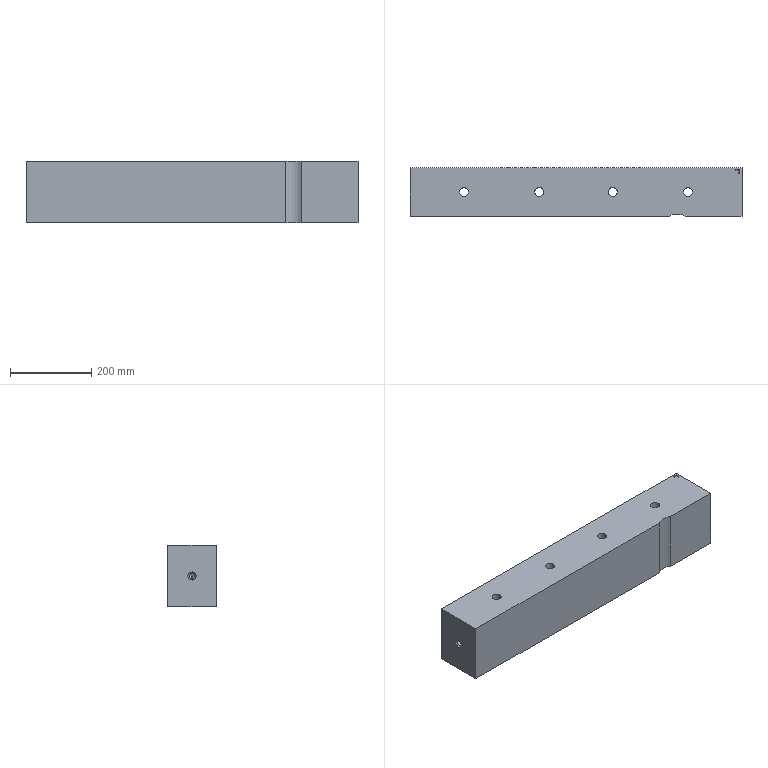Part | Creo | 1 solid | 43 faces | box 815 x 120 x 150 mm | volume 14398522 mm3 | cylinder 17 | plane 14 | cone 12 | commonest cylinder face diameters 22 x8 12 x4 14 x4 68 x1
STEP:
#1=CARTESIAN_POINT('',(0.,0.,0.));
#2=DIRECTION('',(0.,0.,1.));
#3=DIRECTION('',(1.,0.,0.));
#4=AXIS2_PLACEMENT_3D('',#1,#2,#3);
#5=CARTESIAN_POINT('',(300.814,185.373,-228.441));
#6=VERTEX_POINT('',#5);
#7=CARTESIAN_POINT('',(300.814,185.373,-378.441));
#8=VERTEX_POINT('',#7);
#9=CARTESIAN_POINT('',(300.814,185.373,-228.441));
#10=DIRECTION('',(0.,0.,-1.));
#11=VECTOR('',#10,150.);
#12=LINE('',#9,#11);
#13=EDGE_CURVE('',#6,#8,#12,.T.);
#14=ORIENTED_EDGE('',*,*,#13,.T.);
#15=CARTESIAN_POINT('',(-335.899,185.373,-378.441));
#16=VERTEX_POINT('',#15);
#17=CARTESIAN_POINT('',(-335.899,185.373,-378.441));
#18=DIRECTION('',(1.,0.,0.));
#19=VECTOR('',#18,636.713);
#20=LINE('',#17,#19);
#21=EDGE_CURVE('',#16,#8,#20,.T.);
#22=ORIENTED_EDGE('',*,*,#21,.F.);
#23=CARTESIAN_POINT('',(-335.899,185.373,-228.441));
#24=VERTEX_POINT('',#23);
#25=CARTESIAN_POINT('',(-335.899,185.373,-228.441));
#26=DIRECTION('',(0.,0.,-1.));
#27=VECTOR('',#26,150.);
#28=LINE('',#25,#27);
#29=EDGE_CURVE('',#24,#16,#28,.T.);
#30=ORIENTED_EDGE('',*,*,#29,.F.);
#31=CARTESIAN_POINT('',(-335.899,185.373,-228.441));
#32=DIRECTION('',(1.,0.,0.));
#33=VECTOR('',#32,636.713);
#34=LINE('',#31,#33);
#35=EDGE_CURVE('',#24,#6,#34,.T.);
#36=ORIENTED_EDGE('',*,*,#35,.T.);
#37=EDGE_LOOP('',(#14,#22,#30,#36));
#38=FACE_OUTER_BOUND('',#37,.F.);
#39=CARTESIAN_POINT('',(464.101,185.373,-378.441));
#40=DIRECTION('',(0.,1.,0.));
#41=DIRECTION('',(-1.,0.,0.));
#42=AXIS2_PLACEMENT_3D('',#39,#40,#41);
#43=PLANE('',#42);
#44=ADVANCED_FACE('',(#38),#43,.F.);
#45=CARTESIAN_POINT('',(339.388,185.373,-378.441));
#46=VERTEX_POINT('',#45);
#47=CARTESIAN_POINT('',(320.101,157.373,-378.441));
#48=DIRECTION('',(0.,0.,1.));
#49=DIRECTION('',(0.5673,0.8235,0.));
#50=AXIS2_PLACEMENT_3D('',#47,#48,#49);
#51=CIRCLE('',#50,34.);
#52=EDGE_CURVE('',#46,#8,#51,.T.);
#53=ORIENTED_EDGE('',*,*,#52,.T.);
#54=ORIENTED_EDGE('',*,*,#13,.F.);
#55=CARTESIAN_POINT('',(339.388,185.373,-228.441));
#56=VERTEX_POINT('',#55);
#57=CARTESIAN_POINT('',(320.101,157.373,-228.441));
#58=DIRECTION('',(0.,0.,-1.));
#59=DIRECTION('',(-0.5673,0.8235,0.));
#60=AXIS2_PLACEMENT_3D('',#57,#58,#59);
#61=CIRCLE('',#60,34.);
#62=EDGE_CURVE('',#6,#56,#61,.T.);
#63=ORIENTED_EDGE('',*,*,#62,.T.);
#64=CARTESIAN_POINT('',(339.388,185.373,-378.441));
#65=DIRECTION('',(0.,0.,1.));
#66=VECTOR('',#65,150.);
#67=LINE('',#64,#66);
#68=EDGE_CURVE('',#46,#56,#67,.T.);
#69=ORIENTED_EDGE('',*,*,#68,.F.);
#70=EDGE_LOOP('',(#53,#54,#63,#69));
#71=FACE_OUTER_BOUND('',#70,.F.);
#72=CARTESIAN_POINT('',(320.101,157.373,-453.441));
#73=DIRECTION('',(0.,0.,1.));
#74=DIRECTION('',(1.,0.,0.));
#75=AXIS2_PLACEMENT_3D('',#72,#73,#74);
#76=CYLINDRICAL_SURFACE('',#75,34.);
#77=ADVANCED_FACE('',(#71),#76,.F.);
#78=ORIENTED_EDGE('',*,*,#52,.F.);
#79=CARTESIAN_POINT('',(479.101,185.373,-378.441));
#80=VERTEX_POINT('',#79);
#81=CARTESIAN_POINT('',(339.388,185.373,-378.441));
#82=DIRECTION('',(1.,0.,0.));
#83=VECTOR('',#82,139.713);
#84=LINE('',#81,#83);
#85=EDGE_CURVE('',#46,#80,#84,.T.);
#86=ORIENTED_EDGE('',*,*,#85,.T.);
#87=CARTESIAN_POINT('',(479.101,305.373,-378.441));
#88=VERTEX_POINT('',#87);
#89=CARTESIAN_POINT('',(479.101,185.373,-378.441));
#90=DIRECTION('',(0.,1.,0.));
#91=VECTOR('',#90,120.);
#92=LINE('',#89,#91);
#93=EDGE_CURVE('',#80,#88,#92,.T.);
#94=ORIENTED_EDGE('',*,*,#93,.T.);
#95=CARTESIAN_POINT('',(-335.899,305.373,-378.441));
#96=VERTEX_POINT('',#95);
#97=CARTESIAN_POINT('',(479.101,305.373,-378.441));
#98=DIRECTION('',(-1.,0.,0.));
#99=VECTOR('',#98,815.);
#100=LINE('',#97,#99);
#101=EDGE_CURVE('',#88,#96,#100,.T.);
#102=ORIENTED_EDGE('',*,*,#101,.T.);
#103=CARTESIAN_POINT('',(-335.899,305.373,-378.441));
#104=DIRECTION('',(0.,-1.,0.));
#105=VECTOR('',#104,120.);
#106=LINE('',#103,#105);
#107=EDGE_CURVE('',#96,#16,#106,.T.);
#108=ORIENTED_EDGE('',*,*,#107,.T.);
#109=ORIENTED_EDGE('',*,*,#21,.T.);
#110=EDGE_LOOP('',(#78,#86,#94,#102,#108,#109));
#111=FACE_OUTER_BOUND('',#110,.F.);
#112=CARTESIAN_POINT('',(426.101,251.373,-378.441));
#113=VERTEX_POINT('',#112);
#114=CARTESIAN_POINT('',(420.101,245.373,-378.441));
#115=VERTEX_POINT('',#114);
#116=CARTESIAN_POINT('',(426.101,245.373,-378.441));
#117=DIRECTION('',(0.,0.,1.));
#118=DIRECTION('',(0.,1.,0.));
#119=AXIS2_PLACEMENT_3D('',#116,#117,#118);
#120=CIRCLE('',#119,6.);
#121=EDGE_CURVE('',#113,#115,#120,.T.);
#122=ORIENTED_EDGE('',*,*,#121,.F.);
#123=CARTESIAN_POINT('',(432.101,245.373,-378.441));
#124=VERTEX_POINT('',#123);
#125=CARTESIAN_POINT('',(426.101,245.373,-378.441));
#126=DIRECTION('',(0.,0.,1.));
#127=DIRECTION('',(1.,0.,0.));
#128=AXIS2_PLACEMENT_3D('',#125,#126,#127);
#129=CIRCLE('',#128,6.);
#130=EDGE_CURVE('',#124,#113,#129,.T.);
#131=ORIENTED_EDGE('',*,*,#130,.F.);
#132=CARTESIAN_POINT('',(426.101,239.373,-378.441));
#133=VERTEX_POINT('',#132);
#134=CARTESIAN_POINT('',(426.101,245.373,-378.441));
#135=DIRECTION('',(0.,0.,1.));
#136=DIRECTION('',(0.,-1.,0.));
#137=AXIS2_PLACEMENT_3D('',#134,#135,#136);
#138=CIRCLE('',#137,6.);
#139=EDGE_CURVE('',#133,#124,#138,.T.);
#140=ORIENTED_EDGE('',*,*,#139,.F.);
#141=CARTESIAN_POINT('',(426.101,245.373,-378.441));
#142=DIRECTION('',(0.,0.,1.));
#143=DIRECTION('',(-1.,0.,0.));
#144=AXIS2_PLACEMENT_3D('',#141,#142,#143);
#145=CIRCLE('',#144,6.);
#146=EDGE_CURVE('',#115,#133,#145,.T.);
#147=ORIENTED_EDGE('',*,*,#146,.F.);
#148=EDGE_LOOP('',(#122,#131,#140,#147));
#149=FACE_BOUND('',#148,.F.);
#150=CARTESIAN_POINT('',(-203.399,256.373,-378.441));
#151=VERTEX_POINT('',#150);
#152=CARTESIAN_POINT('',(-214.399,245.373,-378.441));
#153=VERTEX_POINT('',#152);
#154=CARTESIAN_POINT('',(-203.399,245.373,-378.441));
#155=DIRECTION('',(0.,0.,1.));
#156=DIRECTION('',(0.,1.,0.));
#157=AXIS2_PLACEMENT_3D('',#154,#155,#156);
#158=CIRCLE('',#157,11.);
#159=EDGE_CURVE('',#151,#153,#158,.T.);
#160=ORIENTED_EDGE('',*,*,#159,.F.);
#161=CARTESIAN_POINT('',(-192.399,245.373,-378.441));
#162=VERTEX_POINT('',#161);
#163=CARTESIAN_POINT('',(-203.399,245.373,-378.441));
#164=DIRECTION('',(0.,0.,1.));
#165=DIRECTION('',(1.,0.,0.));
#166=AXIS2_PLACEMENT_3D('',#163,#164,#165);
#167=CIRCLE('',#166,11.);
#168=EDGE_CURVE('',#162,#151,#167,.T.);
#169=ORIENTED_EDGE('',*,*,#168,.F.);
#170=CARTESIAN_POINT('',(-203.399,234.373,-378.441));
#171=VERTEX_POINT('',#170);
#172=CARTESIAN_POINT('',(-203.399,245.373,-378.441));
#173=DIRECTION('',(0.,0.,1.));
#174=DIRECTION('',(0.,-1.,0.));
#175=AXIS2_PLACEMENT_3D('',#172,#173,#174);
#176=CIRCLE('',#175,11.);
#177=EDGE_CURVE('',#171,#162,#176,.T.);
#178=ORIENTED_EDGE('',*,*,#177,.F.);
#179=CARTESIAN_POINT('',(-203.399,245.373,-378.441));
#180=DIRECTION('',(0.,0.,1.));
#181=DIRECTION('',(-1.,0.,0.));
#182=AXIS2_PLACEMENT_3D('',#179,#180,#181);
#183=CIRCLE('',#182,11.);
#184=EDGE_CURVE('',#153,#171,#183,.T.);
#185=ORIENTED_EDGE('',*,*,#184,.F.);
#186=EDGE_LOOP('',(#160,#169,#178,#185));
#187=FACE_BOUND('',#186,.F.);
#188=CARTESIAN_POINT('',(346.601,256.373,-378.441));
#189=VERTEX_POINT('',#188);
#190=CARTESIAN_POINT('',(335.601,245.373,-378.441));
#191=VERTEX_POINT('',#190);
#192=CARTESIAN_POINT('',(346.601,245.373,-378.441));
#193=DIRECTION('',(0.,0.,1.));
#194=DIRECTION('',(0.,1.,0.));
#195=AXIS2_PLACEMENT_3D('',#192,#193,#194);
#196=CIRCLE('',#195,11.);
#197=EDGE_CURVE('',#189,#191,#196,.T.);
#198=ORIENTED_EDGE('',*,*,#197,.F.);
#199=CARTESIAN_POINT('',(357.601,245.373,-378.441));
#200=VERTEX_POINT('',#199);
#201=CARTESIAN_POINT('',(346.601,245.373,-378.441));
#202=DIRECTION('',(0.,0.,1.));
#203=DIRECTION('',(1.,0.,0.));
#204=AXIS2_PLACEMENT_3D('',#201,#202,#203);
#205=CIRCLE('',#204,11.);
#206=EDGE_CURVE('',#200,#189,#205,.T.);
#207=ORIENTED_EDGE('',*,*,#206,.F.);
#208=CARTESIAN_POINT('',(346.601,234.373,-378.441));
#209=VERTEX_POINT('',#208);
#210=CARTESIAN_POINT('',(346.601,245.373,-378.441));
#211=DIRECTION('',(0.,0.,1.));
#212=DIRECTION('',(0.,-1.,0.));
#213=AXIS2_PLACEMENT_3D('',#210,#211,#212);
#214=CIRCLE('',#213,11.);
#215=EDGE_CURVE('',#209,#200,#214,.T.);
#216=ORIENTED_EDGE('',*,*,#215,.F.);
#217=CARTESIAN_POINT('',(346.601,245.373,-378.441));
#218=DIRECTION('',(0.,0.,1.));
#219=DIRECTION('',(-1.,0.,0.));
#220=AXIS2_PLACEMENT_3D('',#217,#218,#219);
#221=CIRCLE('',#220,11.);
#222=EDGE_CURVE('',#191,#209,#221,.T.);
#223=ORIENTED_EDGE('',*,*,#222,.F.);
#224=EDGE_LOOP('',(#198,#207,#216,#223));
#225=FACE_BOUND('',#224,.F.);
#226=CARTESIAN_POINT('',(-18.399,256.373,-378.441));
#227=VERTEX_POINT('',#226);
#228=CARTESIAN_POINT('',(-29.399,245.373,-378.441));
#229=VERTEX_POINT('',#228);
#230=CARTESIAN_POINT('',(-18.399,245.373,-378.441));
#231=DIRECTION('',(0.,0.,1.));
#232=DIRECTION('',(0.,1.,0.));
#233=AXIS2_PLACEMENT_3D('',#230,#231,#232);
#234=CIRCLE('',#233,11.);
#235=EDGE_CURVE('',#227,#229,#234,.T.);
#236=ORIENTED_EDGE('',*,*,#235,.F.);
#237=CARTESIAN_POINT('',(-7.399,245.373,-378.441));
#238=VERTEX_POINT('',#237);
#239=CARTESIAN_POINT('',(-18.399,245.373,-378.441));
#240=DIRECTION('',(0.,0.,1.));
#241=DIRECTION('',(1.,0.,0.));
#242=AXIS2_PLACEMENT_3D('',#239,#240,#241);
#243=CIRCLE('',#242,11.);
#244=EDGE_CURVE('',#238,#227,#243,.T.);
#245=ORIENTED_EDGE('',*,*,#244,.F.);
#246=CARTESIAN_POINT('',(-18.399,234.373,-378.441));
#247=VERTEX_POINT('',#246);
#248=CARTESIAN_POINT('',(-18.399,245.373,-378.441));
#249=DIRECTION('',(0.,0.,1.));
#250=DIRECTION('',(0.,-1.,0.));
#251=AXIS2_PLACEMENT_3D('',#248,#249,#250);
#252=CIRCLE('',#251,11.);
#253=EDGE_CURVE('',#247,#238,#252,.T.);
#254=ORIENTED_EDGE('',*,*,#253,.F.);
#255=CARTESIAN_POINT('',(-18.399,245.373,-378.441));
#256=DIRECTION('',(0.,0.,1.));
#257=DIRECTION('',(-1.,0.,0.));
#258=AXIS2_PLACEMENT_3D('',#255,#256,#257);
#259=CIRCLE('',#258,11.);
#260=EDGE_CURVE('',#229,#247,#259,.T.);
#261=ORIENTED_EDGE('',*,*,#260,.F.);
#262=EDGE_LOOP('',(#236,#245,#254,#261));
#263=FACE_BOUND('',#262,.F.);
#264=CARTESIAN_POINT('',(161.601,256.373,-378.441));
#265=VERTEX_POINT('',#264);
#266=CARTESIAN_POINT('',(150.601,245.373,-378.441));
#267=VERTEX_POINT('',#266);
#268=CARTESIAN_POINT('',(161.601,245.373,-378.441));
#269=DIRECTION('',(0.,0.,1.));
#270=DIRECTION('',(0.,1.,0.));
#271=AXIS2_PLACEMENT_3D('',#268,#269,#270);
#272=CIRCLE('',#271,11.);
#273=EDGE_CURVE('',#265,#267,#272,.T.);
#274=ORIENTED_EDGE('',*,*,#273,.F.);
#275=CARTESIAN_POINT('',(172.601,245.373,-378.441));
#276=VERTEX_POINT('',#275);
#277=CARTESIAN_POINT('',(161.601,245.373,-378.441));
#278=DIRECTION('',(0.,0.,1.));
#279=DIRECTION('',(1.,0.,0.));
#280=AXIS2_PLACEMENT_3D('',#277,#278,#279);
#281=CIRCLE('',#280,11.);
#282=EDGE_CURVE('',#276,#265,#281,.T.);
#283=ORIENTED_EDGE('',*,*,#282,.F.);
#284=CARTESIAN_POINT('',(161.601,234.373,-378.441));
#285=VERTEX_POINT('',#284);
#286=CARTESIAN_POINT('',(161.601,245.373,-378.441));
#287=DIRECTION('',(0.,0.,1.));
#288=DIRECTION('',(0.,-1.,0.));
#289=AXIS2_PLACEMENT_3D('',#286,#287,#288);
#290=CIRCLE('',#289,11.);
#291=EDGE_CURVE('',#285,#276,#290,.T.);
#292=ORIENTED_EDGE('',*,*,#291,.F.);
#293=CARTESIAN_POINT('',(161.601,245.373,-378.441));
#294=DIRECTION('',(0.,0.,1.));
#295=DIRECTION('',(-1.,0.,0.));
#296=AXIS2_PLACEMENT_3D('',#293,#294,#295);
#297=CIRCLE('',#296,11.);
#298=EDGE_CURVE('',#267,#285,#297,.T.);
#299=ORIENTED_EDGE('',*,*,#298,.F.);
#300=EDGE_LOOP('',(#274,#283,#292,#299));
#301=FACE_BOUND('',#300,.F.);
#302=CARTESIAN_POINT('',(-282.899,251.373,-378.441));
#303=VERTEX_POINT('',#302);
#304=CARTESIAN_POINT('',(-288.899,245.373,-378.441));
#305=VERTEX_POINT('',#304);
#306=CARTESIAN_POINT('',(-282.899,245.373,-378.441));
#307=DIRECTION('',(0.,0.,1.));
#308=DIRECTION('',(0.,1.,0.));
#309=AXIS2_PLACEMENT_3D('',#306,#307,#308);
#310=CIRCLE('',#309,6.);
#311=EDGE_CURVE('',#303,#305,#310,.T.);
#312=ORIENTED_EDGE('',*,*,#311,.F.);
#313=CARTESIAN_POINT('',(-276.899,245.373,-378.441));
#314=VERTEX_POINT('',#313);
#315=CARTESIAN_POINT('',(-282.899,245.373,-378.441));
#316=DIRECTION('',(0.,0.,1.));
#317=DIRECTION('',(1.,0.,0.));
#318=AXIS2_PLACEMENT_3D('',#315,#316,#317);
#319=CIRCLE('',#318,6.);
#320=EDGE_CURVE('',#314,#303,#319,.T.);
#321=ORIENTED_EDGE('',*,*,#320,.F.);
#322=CARTESIAN_POINT('',(-282.899,239.373,-378.441));
#323=VERTEX_POINT('',#322);
#324=CARTESIAN_POINT('',(-282.899,245.373,-378.441));
#325=DIRECTION('',(0.,0.,1.));
#326=DIRECTION('',(0.,-1.,0.));
#327=AXIS2_PLACEMENT_3D('',#324,#325,#326);
#328=CIRCLE('',#327,6.);
#329=EDGE_CURVE('',#323,#314,#328,.T.);
#330=ORIENTED_EDGE('',*,*,#329,.F.);
#331=CARTESIAN_POINT('',(-282.899,245.373,-378.441));
#332=DIRECTION('',(0.,0.,1.));
#333=DIRECTION('',(-1.,0.,0.));
#334=AXIS2_PLACEMENT_3D('',#331,#332,#333);
#335=CIRCLE('',#334,6.);
#336=EDGE_CURVE('',#305,#323,#335,.T.);
#337=ORIENTED_EDGE('',*,*,#336,.F.);
#338=EDGE_LOOP('',(#312,#321,#330,#337));
#339=FACE_BOUND('',#338,.F.);
#340=CARTESIAN_POINT('',(464.101,305.373,-378.441));
#341=DIRECTION('',(0.,0.,1.));
#342=DIRECTION('',(1.,0.,0.));
#343=AXIS2_PLACEMENT_3D('',#340,#341,#342);
#344=PLANE('',#343);
#345=ADVANCED_FACE('',(#111,#149,#187,#225,#263,#301,#339),#344,.F.);
#346=CARTESIAN_POINT('',(-288.899,245.373,-344.029));
#347=VERTEX_POINT('',#346);
#348=CARTESIAN_POINT('',(-282.899,251.373,-344.029));
#349=VERTEX_POINT('',#348);
#350=CARTESIAN_POINT('',(-282.899,245.373,-344.029));
#351=DIRECTION('',(0.,0.,-1.));
#352=DIRECTION('',(-1.,0.,0.));
#353=AXIS2_PLACEMENT_3D('',#350,#351,#352);
#354=CIRCLE('',#353,6.);
#355=EDGE_CURVE('',#347,#349,#354,.T.);
#356=ORIENTED_EDGE('',*,*,#355,.T.);
#357=CARTESIAN_POINT('',(-276.899,245.373,-344.029));
#358=VERTEX_POINT('',#357);
#359=CARTESIAN_POINT('',(-282.899,245.373,-344.029));
#360=DIRECTION('',(0.,0.,-1.));
#361=DIRECTION('',(0.,1.,0.));
#362=AXIS2_PLACEMENT_3D('',#359,#360,#361);
#363=CIRCLE('',#362,6.);
#364=EDGE_CURVE('',#349,#358,#363,.T.);
#365=ORIENTED_EDGE('',*,*,#364,.T.);
#366=CARTESIAN_POINT('',(-276.899,245.373,-378.441));
#367=DIRECTION('',(0.,0.,1.));
#368=VECTOR('',#367,34.413);
#369=LINE('',#366,#368);
#370=EDGE_CURVE('',#314,#358,#369,.T.);
#371=ORIENTED_EDGE('',*,*,#370,.F.);
#372=ORIENTED_EDGE('',*,*,#320,.T.);
#373=ORIENTED_EDGE('',*,*,#311,.T.);
#374=CARTESIAN_POINT('',(-288.899,245.373,-378.441));
#375=DIRECTION('',(0.,0.,1.));
#376=VECTOR('',#375,34.413);
#377=LINE('',#374,#376);
#378=EDGE_CURVE('',#305,#347,#377,.T.);
#379=ORIENTED_EDGE('',*,*,#378,.T.);
#380=EDGE_LOOP('',(#356,#365,#371,#372,#373,#379));
#381=FACE_OUTER_BOUND('',#380,.F.);
#382=CARTESIAN_POINT('',(-282.899,245.373,-378.441));
#383=DIRECTION('',(0.,0.,1.));
#384=DIRECTION('',(1.,0.,0.));
#385=AXIS2_PLACEMENT_3D('',#382,#383,#384);
#386=CYLINDRICAL_SURFACE('',#385,6.);
#387=ADVANCED_FACE('',(#381),#386,.F.);
#388=ORIENTED_EDGE('',*,*,#364,.F.);
#389=ORIENTED_EDGE('',*,*,#355,.F.);
#390=CARTESIAN_POINT('',(-282.899,245.373,-340.423));
#391=VERTEX_POINT('',#390);
#392=CARTESIAN_POINT('',(-282.899,245.373,-340.423));
#393=DIRECTION('',(-0.8572,0.,-0.515));
#394=VECTOR('',#393,7.);
#395=LINE('',#392,#394);
#396=EDGE_CURVE('',#391,#347,#395,.T.);
#397=ORIENTED_EDGE('',*,*,#396,.F.);
#398=CARTESIAN_POINT('',(-282.899,245.373,-340.423));
#399=DIRECTION('',(0.8572,0.,-0.515));
#400=VECTOR('',#399,7.);
#401=LINE('',#398,#400);
#402=EDGE_CURVE('',#391,#358,#401,.T.);
#403=ORIENTED_EDGE('',*,*,#402,.T.);
#404=EDGE_LOOP('',(#388,#389,#397,#403));
#405=FACE_OUTER_BOUND('',#404,.F.);
#406=CARTESIAN_POINT('',(-282.899,245.373,-342.485));
#407=DIRECTION('',(0.,0.,-1.));
#408=DIRECTION('',(-1.,0.,0.));
#409=AXIS2_PLACEMENT_3D('',#406,#407,#408);
#410=CONICAL_SURFACE('',#409,3.431,59.);
#411=ADVANCED_FACE('',(#405),#410,.F.);
#412=CARTESIAN_POINT('',(-282.899,245.373,-344.029));
#413=DIRECTION('',(0.,0.,-1.));
#414=DIRECTION('',(1.,0.,0.));
#415=AXIS2_PLACEMENT_3D('',#412,#413,#414);
#416=CIRCLE('',#415,6.);
#417=EDGE_CURVE('',#358,#347,#416,.T.);
#418=ORIENTED_EDGE('',*,*,#417,.F.);
#419=ORIENTED_EDGE('',*,*,#402,.F.);
#420=ORIENTED_EDGE('',*,*,#396,.T.);
#421=EDGE_LOOP('',(#418,#419,#420));
#422=FACE_OUTER_BOUND('',#421,.F.);
#423=CARTESIAN_POINT('',(-282.899,245.373,-342.485));
#424=DIRECTION('',(0.,0.,-1.));
#425=DIRECTION('',(-1.,0.,0.));
#426=AXIS2_PLACEMENT_3D('',#423,#424,#425);
#427=CONICAL_SURFACE('',#426,3.431,59.);
#428=ADVANCED_FACE('',(#422),#427,.F.);
#429=ORIENTED_EDGE('',*,*,#417,.T.);
#430=ORIENTED_EDGE('',*,*,#378,.F.);
#431=ORIENTED_EDGE('',*,*,#336,.T.);
#432=ORIENTED_EDGE('',*,*,#329,.T.);
#433=ORIENTED_EDGE('',*,*,#370,.T.);
#434=EDGE_LOOP('',(#429,#430,#431,#432,#433));
#435=FACE_OUTER_BOUND('',#434,.F.);
#436=CARTESIAN_POINT('',(-282.899,245.373,-378.441));
#437=DIRECTION('',(0.,0.,1.));
#438=DIRECTION('',(1.,0.,0.));
#439=AXIS2_PLACEMENT_3D('',#436,#437,#438);
#440=CYLINDRICAL_SURFACE('',#439,6.);
#441=ADVANCED_FACE('',(#435),#440,.F.);
#442=CARTESIAN_POINT('',(420.101,245.373,-344.029));
#443=VERTEX_POINT('',#442);
#444=CARTESIAN_POINT('',(426.101,251.373,-344.029));
#445=VERTEX_POINT('',#444);
#446=CARTESIAN_POINT('',(426.101,245.373,-344.029));
#447=DIRECTION('',(0.,0.,-1.));
#448=DIRECTION('',(-1.,0.,0.));
#449=AXIS2_PLACEMENT_3D('',#446,#447,#448);
#450=CIRCLE('',#449,6.);
#451=EDGE_CURVE('',#443,#445,#450,.T.);
#452=ORIENTED_EDGE('',*,*,#451,.T.);
#453=CARTESIAN_POINT('',(432.101,245.373,-344.029));
#454=VERTEX_POINT('',#453);
#455=CARTESIAN_POINT('',(426.101,245.373,-344.029));
#456=DIRECTION('',(0.,0.,-1.));
#457=DIRECTION('',(0.,1.,0.));
#458=AXIS2_PLACEMENT_3D('',#455,#456,#457);
#459=CIRCLE('',#458,6.);
#460=EDGE_CURVE('',#445,#454,#459,.T.);
#461=ORIENTED_EDGE('',*,*,#460,.T.);
#462=CARTESIAN_POINT('',(432.101,245.373,-378.441));
#463=DIRECTION('',(0.,0.,1.));
#464=VECTOR('',#463,34.413);
#465=LINE('',#462,#464);
#466=EDGE_CURVE('',#124,#454,#465,.T.);
#467=ORIENTED_EDGE('',*,*,#466,.F.);
#468=ORIENTED_EDGE('',*,*,#130,.T.);
#469=ORIENTED_EDGE('',*,*,#121,.T.);
#470=CARTESIAN_POINT('',(420.101,245.373,-378.441));
#471=DIRECTION('',(0.,0.,1.));
#472=VECTOR('',#471,34.413);
#473=LINE('',#470,#472);
#474=EDGE_CURVE('',#115,#443,#473,.T.);
#475=ORIENTED_EDGE('',*,*,#474,.T.);
#476=EDGE_LOOP('',(#452,#461,#467,#468,#469,#475));
#477=FACE_OUTER_BOUND('',#476,.F.);
#478=CARTESIAN_POINT('',(426.101,245.373,-378.441));
#479=DIRECTION('',(0.,0.,1.));
#480=DIRECTION('',(1.,0.,0.));
#481=AXIS2_PLACEMENT_3D('',#478,#479,#480);
#482=CYLINDRICAL_SURFACE('',#481,6.);
#483=ADVANCED_FACE('',(#477),#482,.F.);
#484=ORIENTED_EDGE('',*,*,#460,.F.);
#485=ORIENTED_EDGE('',*,*,#451,.F.);
#486=CARTESIAN_POINT('',(426.101,245.373,-340.423));
#487=VERTEX_POINT('',#486);
#488=CARTESIAN_POINT('',(426.101,245.373,-340.423));
#489=DIRECTION('',(-0.8572,0.,-0.515));
#490=VECTOR('',#489,7.);
#491=LINE('',#488,#490);
#492=EDGE_CURVE('',#487,#443,#491,.T.);
#493=ORIENTED_EDGE('',*,*,#492,.F.);
#494=CARTESIAN_POINT('',(426.101,245.373,-340.423));
#495=DIRECTION('',(0.8572,0.,-0.515));
#496=VECTOR('',#495,7.);
#497=LINE('',#494,#496);
#498=EDGE_CURVE('',#487,#454,#497,.T.);
#499=ORIENTED_EDGE('',*,*,#498,.T.);
#500=EDGE_LOOP('',(#484,#485,#493,#499));
#501=FACE_OUTER_BOUND('',#500,.F.);
#502=CARTESIAN_POINT('',(426.101,245.373,-342.485));
#503=DIRECTION('',(0.,0.,-1.));
#504=DIRECTION('',(-1.,0.,0.));
#505=AXIS2_PLACEMENT_3D('',#502,#503,#504);
#506=CONICAL_SURFACE('',#505,3.431,59.);
#507=ADVANCED_FACE('',(#501),#506,.F.);
#508=CARTESIAN_POINT('',(426.101,245.373,-344.029));
#509=DIRECTION('',(0.,0.,-1.));
#510=DIRECTION('',(1.,0.,0.));
#511=AXIS2_PLACEMENT_3D('',#508,#509,#510);
#512=CIRCLE('',#511,6.);
#513=EDGE_CURVE('',#454,#443,#512,.T.);
#514=ORIENTED_EDGE('',*,*,#513,.F.);
#515=ORIENTED_EDGE('',*,*,#498,.F.);
#516=ORIENTED_EDGE('',*,*,#492,.T.);
#517=EDGE_LOOP('',(#514,#515,#516));
#518=FACE_OUTER_BOUND('',#517,.F.);
#519=CARTESIAN_POINT('',(426.101,245.373,-342.485));
#520=DIRECTION('',(0.,0.,-1.));
#521=DIRECTION('',(-1.,0.,0.));
#522=AXIS2_PLACEMENT_3D('',#519,#520,#521);
#523=CONICAL_SURFACE('',#522,3.431,59.);
#524=ADVANCED_FACE('',(#518),#523,.F.);
#525=ORIENTED_EDGE('',*,*,#513,.T.);
#526=ORIENTED_EDGE('',*,*,#474,.F.);
#527=ORIENTED_EDGE('',*,*,#146,.T.);
#528=ORIENTED_EDGE('',*,*,#139,.T.);
#529=ORIENTED_EDGE('',*,*,#466,.T.);
#530=EDGE_LOOP('',(#525,#526,#527,#528,#529));
#531=FACE_OUTER_BOUND('',#530,.F.);
#532=CARTESIAN_POINT('',(426.101,245.373,-378.441));
#533=DIRECTION('',(0.,0.,1.));
#534=DIRECTION('',(1.,0.,0.));
#535=AXIS2_PLACEMENT_3D('',#532,#533,#534);
#536=CYLINDRICAL_SURFACE('',#535,6.);
#537=ADVANCED_FACE('',(#531),#536,.F.);
#538=CARTESIAN_POINT('',(-214.399,245.373,-228.441));
#539=VERTEX_POINT('',#538);
#540=CARTESIAN_POINT('',(-203.399,256.373,-228.441));
#541=VERTEX_POINT('',#540);
#542=CARTESIAN_POINT('',(-203.399,245.373,-228.441));
#543=DIRECTION('',(0.,0.,-1.));
#544=DIRECTION('',(-1.,0.,0.));
#545=AXIS2_PLACEMENT_3D('',#542,#543,#544);
#546=CIRCLE('',#545,11.);
#547=EDGE_CURVE('',#539,#541,#546,.T.);
#548=ORIENTED_EDGE('',*,*,#547,.T.);
#549=CARTESIAN_POINT('',(-192.399,245.373,-228.441));
#550=VERTEX_POINT('',#549);
#551=CARTESIAN_POINT('',(-203.399,245.373,-228.441));
#552=DIRECTION('',(0.,0.,-1.));
#553=DIRECTION('',(0.,1.,0.));
#554=AXIS2_PLACEMENT_3D('',#551,#552,#553);
#555=CIRCLE('',#554,11.);
#556=EDGE_CURVE('',#541,#550,#555,.T.);
#557=ORIENTED_EDGE('',*,*,#556,.T.);
#558=CARTESIAN_POINT('',(-192.399,245.373,-378.441));
#559=DIRECTION('',(0.,0.,1.));
#560=VECTOR('',#559,150.);
#561=LINE('',#558,#560);
#562=EDGE_CURVE('',#162,#550,#561,.T.);
#563=ORIENTED_EDGE('',*,*,#562,.F.);
#564=ORIENTED_EDGE('',*,*,#168,.T.);
#565=ORIENTED_EDGE('',*,*,#159,.T.);
#566=CARTESIAN_POINT('',(-214.399,245.373,-378.441));
#567=DIRECTION('',(0.,0.,1.));
#568=VECTOR('',#567,150.);
#569=LINE('',#566,#568);
#570=EDGE_CURVE('',#153,#539,#569,.T.);
#571=ORIENTED_EDGE('',*,*,#570,.T.);
#572=EDGE_LOOP('',(#548,#557,#563,#564,#565,#571));
#573=FACE_OUTER_BOUND('',#572,.F.);
#574=CARTESIAN_POINT('',(-203.399,245.373,-378.441));
#575=DIRECTION('',(0.,0.,1.));
#576=DIRECTION('',(1.,0.,0.));
#577=AXIS2_PLACEMENT_3D('',#574,#575,#576);
#578=CYLINDRICAL_SURFACE('',#577,11.);
#579=ADVANCED_FACE('',(#573),#578,.F.);
#580=ORIENTED_EDGE('',*,*,#35,.F.);
#581=CARTESIAN_POINT('',(-335.899,305.373,-228.441));
#582=VERTEX_POINT('',#581);
#583=CARTESIAN_POINT('',(-335.899,305.373,-228.441));
#584=DIRECTION('',(0.,-1.,0.));
#585=VECTOR('',#584,120.);
#586=LINE('',#583,#585);
#587=EDGE_CURVE('',#582,#24,#586,.T.);
#588=ORIENTED_EDGE('',*,*,#587,.F.);
#589=CARTESIAN_POINT('',(479.101,305.373,-228.441));
#590=VERTEX_POINT('',#589);
#591=CARTESIAN_POINT('',(479.101,305.373,-228.441));
#592=DIRECTION('',(-1.,0.,0.));
#593=VECTOR('',#592,815.);
#594=LINE('',#591,#593);
#595=EDGE_CURVE('',#590,#582,#594,.T.);
#596=ORIENTED_EDGE('',*,*,#595,.F.);
#597=CARTESIAN_POINT('',(479.101,185.373,-228.441));
#598=VERTEX_POINT('',#597);
#599=CARTESIAN_POINT('',(479.101,185.373,-228.441));
#600=DIRECTION('',(0.,1.,0.));
#601=VECTOR('',#600,120.);
#602=LINE('',#599,#601);
#603=EDGE_CURVE('',#598,#590,#602,.T.);
#604=ORIENTED_EDGE('',*,*,#603,.F.);
#605=CARTESIAN_POINT('',(339.388,185.373,-228.441));
#606=DIRECTION('',(1.,0.,0.));
#607=VECTOR('',#606,139.713);
#608=LINE('',#605,#607);
#609=EDGE_CURVE('',#56,#598,#608,.T.);
#610=ORIENTED_EDGE('',*,*,#609,.F.);
#611=ORIENTED_EDGE('',*,*,#62,.F.);
#612=EDGE_LOOP('',(#580,#588,#596,#604,#610,#611));
#613=FACE_OUTER_BOUND('',#612,.F.);
#614=CARTESIAN_POINT('',(346.601,256.373,-228.441));
#615=VERTEX_POINT('',#614);
#616=CARTESIAN_POINT('',(357.601,245.373,-228.441));
#617=VERTEX_POINT('',#616);
#618=CARTESIAN_POINT('',(346.601,245.373,-228.441));
#619=DIRECTION('',(0.,0.,-1.));
#620=DIRECTION('',(0.,1.,0.));
#621=AXIS2_PLACEMENT_3D('',#618,#619,#620);
#622=CIRCLE('',#621,11.);
#623=EDGE_CURVE('',#615,#617,#622,.T.);
#624=ORIENTED_EDGE('',*,*,#623,.F.);
#625=CARTESIAN_POINT('',(335.601,245.373,-228.441));
#626=VERTEX_POINT('',#625);
#627=CARTESIAN_POINT('',(346.601,245.373,-228.441));
#628=DIRECTION('',(0.,0.,-1.));
#629=DIRECTION('',(-1.,0.,0.));
#630=AXIS2_PLACEMENT_3D('',#627,#628,#629);
#631=CIRCLE('',#630,11.);
#632=EDGE_CURVE('',#626,#615,#631,.T.);
#633=ORIENTED_EDGE('',*,*,#632,.F.);
#634=CARTESIAN_POINT('',(346.601,245.373,-228.441));
#635=DIRECTION('',(0.,0.,-1.));
#636=DIRECTION('',(1.,0.,0.));
#637=AXIS2_PLACEMENT_3D('',#634,#635,#636);
#638=CIRCLE('',#637,11.);
#639=EDGE_CURVE('',#617,#626,#638,.T.);
#640=ORIENTED_EDGE('',*,*,#639,.F.);
#641=EDGE_LOOP('',(#624,#633,#640));
#642=FACE_BOUND('',#641,.F.);
#643=CARTESIAN_POINT('',(-18.399,256.373,-228.441));
#644=VERTEX_POINT('',#643);
#645=CARTESIAN_POINT('',(-7.399,245.373,-228.441));
#646=VERTEX_POINT('',#645);
#647=CARTESIAN_POINT('',(-18.399,245.373,-228.441));
#648=DIRECTION('',(0.,0.,-1.));
#649=DIRECTION('',(0.,1.,0.));
#650=AXIS2_PLACEMENT_3D('',#647,#648,#649);
#651=CIRCLE('',#650,11.);
#652=EDGE_CURVE('',#644,#646,#651,.T.);
#653=ORIENTED_EDGE('',*,*,#652,.F.);
#654=CARTESIAN_POINT('',(-29.399,245.373,-228.441));
#655=VERTEX_POINT('',#654);
#656=CARTESIAN_POINT('',(-18.399,245.373,-228.441));
#657=DIRECTION('',(0.,0.,-1.));
#658=DIRECTION('',(-1.,0.,0.));
#659=AXIS2_PLACEMENT_3D('',#656,#657,#658);
#660=CIRCLE('',#659,11.);
#661=EDGE_CURVE('',#655,#644,#660,.T.);
#662=ORIENTED_EDGE('',*,*,#661,.F.);
#663=CARTESIAN_POINT('',(-18.399,245.373,-228.441));
#664=DIRECTION('',(0.,0.,-1.));
#665=DIRECTION('',(1.,0.,0.));
#666=AXIS2_PLACEMENT_3D('',#663,#664,#665);
#667=CIRCLE('',#666,11.);
#668=EDGE_CURVE('',#646,#655,#667,.T.);
#669=ORIENTED_EDGE('',*,*,#668,.F.);
#670=EDGE_LOOP('',(#653,#662,#669));
#671=FACE_BOUND('',#670,.F.);
#672=CARTESIAN_POINT('',(161.601,256.373,-228.441));
#673=VERTEX_POINT('',#672);
#674=CARTESIAN_POINT('',(172.601,245.373,-228.441));
#675=VERTEX_POINT('',#674);
#676=CARTESIAN_POINT('',(161.601,245.373,-228.441));
#677=DIRECTION('',(0.,0.,-1.));
#678=DIRECTION('',(0.,1.,0.));
#679=AXIS2_PLACEMENT_3D('',#676,#677,#678);
#680=CIRCLE('',#679,11.);
#681=EDGE_CURVE('',#673,#675,#680,.T.);
#682=ORIENTED_EDGE('',*,*,#681,.F.);
#683=CARTESIAN_POINT('',(150.601,245.373,-228.441));
#684=VERTEX_POINT('',#683);
#685=CARTESIAN_POINT('',(161.601,245.373,-228.441));
#686=DIRECTION('',(0.,0.,-1.));
#687=DIRECTION('',(-1.,0.,0.));
#688=AXIS2_PLACEMENT_3D('',#685,#686,#687);
#689=CIRCLE('',#688,11.);
#690=EDGE_CURVE('',#684,#673,#689,.T.);
#691=ORIENTED_EDGE('',*,*,#690,.F.);
#692=CARTESIAN_POINT('',(161.601,245.373,-228.441));
#693=DIRECTION('',(0.,0.,-1.));
#694=DIRECTION('',(1.,0.,0.));
#695=AXIS2_PLACEMENT_3D('',#692,#693,#694);
#696=CIRCLE('',#695,11.);
#697=EDGE_CURVE('',#675,#684,#696,.T.);
#698=ORIENTED_EDGE('',*,*,#697,.F.);
#699=EDGE_LOOP('',(#682,#691,#698));
#700=FACE_BOUND('',#699,.F.);
#701=CARTESIAN_POINT('',(464.101,300.373,-228.441));
#702=VERTEX_POINT('',#701);
#703=CARTESIAN_POINT('',(474.101,300.373,-228.441));
#704=VERTEX_POINT('',#703);
#705=CARTESIAN_POINT('',(464.101,300.373,-228.441));
#706=DIRECTION('',(1.,0.,0.));
#707=VECTOR('',#706,10.);
#708=LINE('',#705,#707);
#709=EDGE_CURVE('',#702,#704,#708,.T.);
#710=ORIENTED_EDGE('',*,*,#709,.F.);
#711=CARTESIAN_POINT('',(464.101,297.373,-228.441));
#712=VERTEX_POINT('',#711);
#713=CARTESIAN_POINT('',(464.101,297.373,-228.441));
#714=DIRECTION('',(0.,1.,0.));
#715=VECTOR('',#714,3.);
#716=LINE('',#713,#715);
#717=EDGE_CURVE('',#712,#702,#716,.T.);
#718=ORIENTED_EDGE('',*,*,#717,.F.);
#719=CARTESIAN_POINT('',(471.101,297.373,-228.441));
#720=VERTEX_POINT('',#719);
#721=CARTESIAN_POINT('',(471.101,297.373,-228.441));
#722=DIRECTION('',(-1.,0.,0.));
#723=VECTOR('',#722,7.);
#724=LINE('',#721,#723);
#725=EDGE_CURVE('',#720,#712,#724,.T.);
#726=ORIENTED_EDGE('',*,*,#725,.F.);
#727=CARTESIAN_POINT('',(471.101,290.373,-228.441));
#728=VERTEX_POINT('',#727);
#729=CARTESIAN_POINT('',(471.101,290.373,-228.441));
#730=DIRECTION('',(0.,1.,0.));
#731=VECTOR('',#730,7.);
#732=LINE('',#729,#731);
#733=EDGE_CURVE('',#728,#720,#732,.T.);
#734=ORIENTED_EDGE('',*,*,#733,.F.);
#735=CARTESIAN_POINT('',(474.101,290.373,-228.441));
#736=VERTEX_POINT('',#735);
#737=CARTESIAN_POINT('',(474.101,290.373,-228.441));
#738=DIRECTION('',(-1.,0.,0.));
#739=VECTOR('',#738,3.);
#740=LINE('',#737,#739);
#741=EDGE_CURVE('',#736,#728,#740,.T.);
#742=ORIENTED_EDGE('',*,*,#741,.F.);
#743=CARTESIAN_POINT('',(474.101,300.373,-228.441));
#744=DIRECTION('',(0.,-1.,0.));
#745=VECTOR('',#744,10.);
#746=LINE('',#743,#745);
#747=EDGE_CURVE('',#704,#736,#746,.T.);
#748=ORIENTED_EDGE('',*,*,#747,.F.);
#749=EDGE_LOOP('',(#710,#718,#726,#734,#742,#748));
#750=FACE_BOUND('',#749,.F.);
#751=ORIENTED_EDGE('',*,*,#556,.F.);
#752=ORIENTED_EDGE('',*,*,#547,.F.);
#753=CARTESIAN_POINT('',(-203.399,245.373,-228.441));
#754=DIRECTION('',(0.,0.,-1.));
#755=DIRECTION('',(1.,0.,0.));
#756=AXIS2_PLACEMENT_3D('',#753,#754,#755);
#757=CIRCLE('',#756,11.);
#758=EDGE_CURVE('',#550,#539,#757,.T.);
#759=ORIENTED_EDGE('',*,*,#758,.F.);
#760=EDGE_LOOP('',(#751,#752,#759));
#761=FACE_BOUND('',#760,.F.);
#762=CARTESIAN_POINT('',(464.101,305.373,-228.441));
#763=DIRECTION('',(0.,0.,1.));
#764=DIRECTION('',(1.,0.,0.));
#765=AXIS2_PLACEMENT_3D('',#762,#763,#764);
#766=PLANE('',#765);
#767=ADVANCED_FACE('',(#613,#642,#671,#700,#750,#761),#766,.T.);
#768=ORIENTED_EDGE('',*,*,#758,.T.);
#769=ORIENTED_EDGE('',*,*,#570,.F.);
#770=ORIENTED_EDGE('',*,*,#184,.T.);
#771=ORIENTED_EDGE('',*,*,#177,.T.);
#772=ORIENTED_EDGE('',*,*,#562,.T.);
#773=EDGE_LOOP('',(#768,#769,#770,#771,#772));
#774=FACE_OUTER_BOUND('',#773,.F.);
#775=CARTESIAN_POINT('',(-203.399,245.373,-378.441));
#776=DIRECTION('',(0.,0.,1.));
#777=DIRECTION('',(1.,0.,0.));
#778=AXIS2_PLACEMENT_3D('',#775,#776,#777);
#779=CYLINDRICAL_SURFACE('',#778,11.);
#780=ADVANCED_FACE('',(#774),#779,.F.);
#781=ORIENTED_EDGE('',*,*,#632,.T.);
#782=ORIENTED_EDGE('',*,*,#623,.T.);
#783=CARTESIAN_POINT('',(357.601,245.373,-378.441));
#784=DIRECTION('',(0.,0.,1.));
#785=VECTOR('',#784,150.);
#786=LINE('',#783,#785);
#787=EDGE_CURVE('',#200,#617,#786,.T.);
#788=ORIENTED_EDGE('',*,*,#787,.F.);
#789=ORIENTED_EDGE('',*,*,#206,.T.);
#790=ORIENTED_EDGE('',*,*,#197,.T.);
#791=CARTESIAN_POINT('',(335.601,245.373,-378.441));
#792=DIRECTION('',(0.,0.,1.));
#793=VECTOR('',#792,150.);
#794=LINE('',#791,#793);
#795=EDGE_CURVE('',#191,#626,#794,.T.);
#796=ORIENTED_EDGE('',*,*,#795,.T.);
#797=EDGE_LOOP('',(#781,#782,#788,#789,#790,#796));
#798=FACE_OUTER_BOUND('',#797,.F.);
#799=CARTESIAN_POINT('',(346.601,245.373,-378.441));
#800=DIRECTION('',(0.,0.,1.));
#801=DIRECTION('',(1.,0.,0.));
#802=AXIS2_PLACEMENT_3D('',#799,#800,#801);
#803=CYLINDRICAL_SURFACE('',#802,11.);
#804=ADVANCED_FACE('',(#798),#803,.F.);
#805=ORIENTED_EDGE('',*,*,#639,.T.);
#806=ORIENTED_EDGE('',*,*,#795,.F.);
#807=ORIENTED_EDGE('',*,*,#222,.T.);
#808=ORIENTED_EDGE('',*,*,#215,.T.);
#809=ORIENTED_EDGE('',*,*,#787,.T.);
#810=EDGE_LOOP('',(#805,#806,#807,#808,#809));
#811=FACE_OUTER_BOUND('',#810,.F.);
#812=CARTESIAN_POINT('',(346.601,245.373,-378.441));
#813=DIRECTION('',(0.,0.,1.));
#814=DIRECTION('',(1.,0.,0.));
#815=AXIS2_PLACEMENT_3D('',#812,#813,#814);
#816=CYLINDRICAL_SURFACE('',#815,11.);
#817=ADVANCED_FACE('',(#811),#816,.F.);
#818=ORIENTED_EDGE('',*,*,#661,.T.);
#819=ORIENTED_EDGE('',*,*,#652,.T.);
#820=CARTESIAN_POINT('',(-7.399,245.373,-378.441));
#821=DIRECTION('',(0.,0.,1.));
#822=VECTOR('',#821,150.);
#823=LINE('',#820,#822);
#824=EDGE_CURVE('',#238,#646,#823,.T.);
#825=ORIENTED_EDGE('',*,*,#824,.F.);
#826=ORIENTED_EDGE('',*,*,#244,.T.);
#827=ORIENTED_EDGE('',*,*,#235,.T.);
#828=CARTESIAN_POINT('',(-29.399,245.373,-378.441));
#829=DIRECTION('',(0.,0.,1.));
#830=VECTOR('',#829,150.);
#831=LINE('',#828,#830);
#832=EDGE_CURVE('',#229,#655,#831,.T.);
#833=ORIENTED_EDGE('',*,*,#832,.T.);
#834=EDGE_LOOP('',(#818,#819,#825,#826,#827,#833));
#835=FACE_OUTER_BOUND('',#834,.F.);
#836=CARTESIAN_POINT('',(-18.399,245.373,-378.441));
#837=DIRECTION('',(0.,0.,1.));
#838=DIRECTION('',(1.,0.,0.));
#839=AXIS2_PLACEMENT_3D('',#836,#837,#838);
#840=CYLINDRICAL_SURFACE('',#839,11.);
#841=ADVANCED_FACE('',(#835),#840,.F.);
#842=ORIENTED_EDGE('',*,*,#668,.T.);
#843=ORIENTED_EDGE('',*,*,#832,.F.);
#844=ORIENTED_EDGE('',*,*,#260,.T.);
#845=ORIENTED_EDGE('',*,*,#253,.T.);
#846=ORIENTED_EDGE('',*,*,#824,.T.);
#847=EDGE_LOOP('',(#842,#843,#844,#845,#846));
#848=FACE_OUTER_BOUND('',#847,.F.);
#849=CARTESIAN_POINT('',(-18.399,245.373,-378.441));
#850=DIRECTION('',(0.,0.,1.));
#851=DIRECTION('',(1.,0.,0.));
#852=AXIS2_PLACEMENT_3D('',#849,#850,#851);
#853=CYLINDRICAL_SURFACE('',#852,11.);
#854=ADVANCED_FACE('',(#848),#853,.F.);
#855=ORIENTED_EDGE('',*,*,#690,.T.);
#856=ORIENTED_EDGE('',*,*,#681,.T.);
#857=CARTESIAN_POINT('',(172.601,245.373,-378.441));
#858=DIRECTION('',(0.,0.,1.));
#859=VECTOR('',#858,150.);
#860=LINE('',#857,#859);
#861=EDGE_CURVE('',#276,#675,#860,.T.);
#862=ORIENTED_EDGE('',*,*,#861,.F.);
#863=ORIENTED_EDGE('',*,*,#282,.T.);
#864=ORIENTED_EDGE('',*,*,#273,.T.);
#865=CARTESIAN_POINT('',(150.601,245.373,-378.441));
#866=DIRECTION('',(0.,0.,1.));
#867=VECTOR('',#866,150.);
#868=LINE('',#865,#867);
#869=EDGE_CURVE('',#267,#684,#868,.T.);
#870=ORIENTED_EDGE('',*,*,#869,.T.);
#871=EDGE_LOOP('',(#855,#856,#862,#863,#864,#870));
#872=FACE_OUTER_BOUND('',#871,.F.);
#873=CARTESIAN_POINT('',(161.601,245.373,-378.441));
#874=DIRECTION('',(0.,0.,1.));
#875=DIRECTION('',(1.,0.,0.));
#876=AXIS2_PLACEMENT_3D('',#873,#874,#875);
#877=CYLINDRICAL_SURFACE('',#876,11.);
#878=ADVANCED_FACE('',(#872),#877,.F.);
#879=ORIENTED_EDGE('',*,*,#697,.T.);
#880=ORIENTED_EDGE('',*,*,#869,.F.);
#881=ORIENTED_EDGE('',*,*,#298,.T.);
#882=ORIENTED_EDGE('',*,*,#291,.T.);
#883=ORIENTED_EDGE('',*,*,#861,.T.);
#884=EDGE_LOOP('',(#879,#880,#881,#882,#883));
#885=FACE_OUTER_BOUND('',#884,.F.);
#886=CARTESIAN_POINT('',(161.601,245.373,-378.441));
#887=DIRECTION('',(0.,0.,1.));
#888=DIRECTION('',(1.,0.,0.));
#889=AXIS2_PLACEMENT_3D('',#886,#887,#888);
#890=CYLINDRICAL_SURFACE('',#889,11.);
#891=ADVANCED_FACE('',(#885),#890,.F.);
#892=ORIENTED_EDGE('',*,*,#709,.T.);
#893=CARTESIAN_POINT('',(474.101,300.373,-231.441));
#894=VERTEX_POINT('',#893);
#895=CARTESIAN_POINT('',(474.101,300.373,-228.441));
#896=DIRECTION('',(0.,0.,-1.));
#897=VECTOR('',#896,3.);
#898=LINE('',#895,#897);
#899=EDGE_CURVE('',#704,#894,#898,.T.);
#900=ORIENTED_EDGE('',*,*,#899,.T.);
#901=CARTESIAN_POINT('',(464.101,300.373,-231.441));
#902=VERTEX_POINT('',#901);
#903=CARTESIAN_POINT('',(464.101,300.373,-231.441));
#904=DIRECTION('',(1.,0.,0.));
#905=VECTOR('',#904,10.);
#906=LINE('',#903,#905);
#907=EDGE_CURVE('',#902,#894,#906,.T.);
#908=ORIENTED_EDGE('',*,*,#907,.F.);
#909=CARTESIAN_POINT('',(464.101,300.373,-228.441));
#910=DIRECTION('',(0.,0.,-1.));
#911=VECTOR('',#910,3.);
#912=LINE('',#909,#911);
#913=EDGE_CURVE('',#702,#902,#912,.T.);
#914=ORIENTED_EDGE('',*,*,#913,.F.);
#915=EDGE_LOOP('',(#892,#900,#908,#914));
#916=FACE_OUTER_BOUND('',#915,.F.);
#917=CARTESIAN_POINT('',(464.101,300.373,-231.441));
#918=DIRECTION('',(0.,1.,0.));
#919=DIRECTION('',(0.,0.,1.));
#920=AXIS2_PLACEMENT_3D('',#917,#918,#919);
#921=PLANE('',#920);
#922=ADVANCED_FACE('',(#916),#921,.F.);
#923=ORIENTED_EDGE('',*,*,#747,.T.);
#924=CARTESIAN_POINT('',(474.101,290.373,-231.441));
#925=VERTEX_POINT('',#924);
#926=CARTESIAN_POINT('',(474.101,290.373,-228.441));
#927=DIRECTION('',(0.,0.,-1.));
#928=VECTOR('',#927,3.);
#929=LINE('',#926,#928);
#930=EDGE_CURVE('',#736,#925,#929,.T.);
#931=ORIENTED_EDGE('',*,*,#930,.T.);
#932=CARTESIAN_POINT('',(474.101,300.373,-231.441));
#933=DIRECTION('',(0.,-1.,0.));
#934=VECTOR('',#933,10.);
#935=LINE('',#932,#934);
#936=EDGE_CURVE('',#894,#925,#935,.T.);
#937=ORIENTED_EDGE('',*,*,#936,.F.);
#938=ORIENTED_EDGE('',*,*,#899,.F.);
#939=EDGE_LOOP('',(#923,#931,#937,#938));
#940=FACE_OUTER_BOUND('',#939,.F.);
#941=CARTESIAN_POINT('',(474.101,305.373,-231.441));
#942=DIRECTION('',(1.,0.,0.));
#943=DIRECTION('',(0.,0.,-1.));
#944=AXIS2_PLACEMENT_3D('',#941,#942,#943);
#945=PLANE('',#944);
#946=ADVANCED_FACE('',(#940),#945,.F.);
#947=ORIENTED_EDGE('',*,*,#741,.T.);
#948=CARTESIAN_POINT('',(471.101,290.373,-231.441));
#949=VERTEX_POINT('',#948);
#950=CARTESIAN_POINT('',(471.101,290.373,-228.441));
#951=DIRECTION('',(0.,0.,-1.));
#952=VECTOR('',#951,3.);
#953=LINE('',#950,#952);
#954=EDGE_CURVE('',#728,#949,#953,.T.);
#955=ORIENTED_EDGE('',*,*,#954,.T.);
#956=CARTESIAN_POINT('',(474.101,290.373,-231.441));
#957=DIRECTION('',(-1.,0.,0.));
#958=VECTOR('',#957,3.);
#959=LINE('',#956,#958);
#960=EDGE_CURVE('',#925,#949,#959,.T.);
#961=ORIENTED_EDGE('',*,*,#960,.F.);
#962=ORIENTED_EDGE('',*,*,#930,.F.);
#963=EDGE_LOOP('',(#947,#955,#961,#962));
#964=FACE_OUTER_BOUND('',#963,.F.);
#965=CARTESIAN_POINT('',(464.101,290.373,-231.441));
#966=DIRECTION('',(0.,-1.,0.));
#967=DIRECTION('',(0.,0.,-1.));
#968=AXIS2_PLACEMENT_3D('',#965,#966,#967);
#969=PLANE('',#968);
#970=ADVANCED_FACE('',(#964),#969,.F.);
#971=ORIENTED_EDGE('',*,*,#733,.T.);
#972=CARTESIAN_POINT('',(471.101,297.373,-231.441));
#973=VERTEX_POINT('',#972);
#974=CARTESIAN_POINT('',(471.101,297.373,-228.441));
#975=DIRECTION('',(0.,0.,-1.));
#976=VECTOR('',#975,3.);
#977=LINE('',#974,#976);
#978=EDGE_CURVE('',#720,#973,#977,.T.);
#979=ORIENTED_EDGE('',*,*,#978,.T.);
#980=CARTESIAN_POINT('',(471.101,290.373,-231.441));
#981=DIRECTION('',(0.,1.,0.));
#982=VECTOR('',#981,7.);
#983=LINE('',#980,#982);
#984=EDGE_CURVE('',#949,#973,#983,.T.);
#985=ORIENTED_EDGE('',*,*,#984,.F.);
#986=ORIENTED_EDGE('',*,*,#954,.F.);
#987=EDGE_LOOP('',(#971,#979,#985,#986));
#988=FACE_OUTER_BOUND('',#987,.F.);
#989=CARTESIAN_POINT('',(471.101,305.373,-231.441));
#990=DIRECTION('',(-1.,0.,0.));
#991=DIRECTION('',(0.,0.,1.));
#992=AXIS2_PLACEMENT_3D('',#989,#990,#991);
#993=PLANE('',#992);
#994=ADVANCED_FACE('',(#988),#993,.F.);
#995=ORIENTED_EDGE('',*,*,#725,.T.);
#996=CARTESIAN_POINT('',(464.101,297.373,-231.441));
#997=VERTEX_POINT('',#996);
#998=CARTESIAN_POINT('',(464.101,297.373,-228.441));
#999=DIRECTION('',(0.,0.,-1.));
#1000=VECTOR('',#999,3.);
#1001=LINE('',#998,#1000);
#1002=EDGE_CURVE('',#712,#997,#1001,.T.);
#1003=ORIENTED_EDGE('',*,*,#1002,.T.);
#1004=CARTESIAN_POINT('',(471.101,297.373,-231.441));
#1005=DIRECTION('',(-1.,0.,0.));
#1006=VECTOR('',#1005,7.);
#1007=LINE('',#1004,#1006);
#1008=EDGE_CURVE('',#973,#997,#1007,.T.);
#1009=ORIENTED_EDGE('',*,*,#1008,.F.);
#1010=ORIENTED_EDGE('',*,*,#978,.F.);
#1011=EDGE_LOOP('',(#995,#1003,#1009,#1010));
#1012=FACE_OUTER_BOUND('',#1011,.F.);
#1013=CARTESIAN_POINT('',(464.101,297.373,-231.441));
#1014=DIRECTION('',(0.,-1.,0.));
#1015=DIRECTION('',(0.,0.,-1.));
#1016=AXIS2_PLACEMENT_3D('',#1013,#1014,#1015);
#1017=PLANE('',#1016);
#1018=ADVANCED_FACE('',(#1012),#1017,.F.);
#1019=ORIENTED_EDGE('',*,*,#717,.T.);
#1020=ORIENTED_EDGE('',*,*,#913,.T.);
#1021=CARTESIAN_POINT('',(464.101,297.373,-231.441));
#1022=DIRECTION('',(0.,1.,0.));
#1023=VECTOR('',#1022,3.);
#1024=LINE('',#1021,#1023);
#1025=EDGE_CURVE('',#997,#902,#1024,.T.);
#1026=ORIENTED_EDGE('',*,*,#1025,.F.);
#1027=ORIENTED_EDGE('',*,*,#1002,.F.);
#1028=EDGE_LOOP('',(#1019,#1020,#1026,#1027));
#1029=FACE_OUTER_BOUND('',#1028,.F.);
#1030=CARTESIAN_POINT('',(464.101,305.373,-231.441));
#1031=DIRECTION('',(-1.,0.,0.));
#1032=DIRECTION('',(0.,0.,1.));
#1033=AXIS2_PLACEMENT_3D('',#1030,#1031,#1032);
#1034=PLANE('',#1033);
#1035=ADVANCED_FACE('',(#1029),#1034,.F.);
#1036=ORIENTED_EDGE('',*,*,#907,.T.);
#1037=ORIENTED_EDGE('',*,*,#936,.T.);
#1038=ORIENTED_EDGE('',*,*,#960,.T.);
#1039=ORIENTED_EDGE('',*,*,#984,.T.);
#1040=ORIENTED_EDGE('',*,*,#1008,.T.);
#1041=ORIENTED_EDGE('',*,*,#1025,.T.);
#1042=EDGE_LOOP('',(#1036,#1037,#1038,#1039,#1040,#1041));
#1043=FACE_OUTER_BOUND('',#1042,.F.);
#1044=CARTESIAN_POINT('',(464.101,305.373,-231.441));
#1045=DIRECTION('',(0.,0.,1.));
#1046=DIRECTION('',(1.,0.,0.));
#1047=AXIS2_PLACEMENT_3D('',#1044,#1045,#1046);
#1048=PLANE('',#1047);
#1049=ADVANCED_FACE('',(#1043),#1048,.T.);
#1050=ORIENTED_EDGE('',*,*,#587,.T.);
#1051=ORIENTED_EDGE('',*,*,#29,.T.);
#1052=ORIENTED_EDGE('',*,*,#107,.F.);
#1053=CARTESIAN_POINT('',(-335.899,305.373,-228.441));
#1054=DIRECTION('',(0.,0.,-1.));
#1055=VECTOR('',#1054,150.);
#1056=LINE('',#1053,#1055);
#1057=EDGE_CURVE('',#582,#96,#1056,.T.);
#1058=ORIENTED_EDGE('',*,*,#1057,.F.);
#1059=EDGE_LOOP('',(#1050,#1051,#1052,#1058));
#1060=FACE_OUTER_BOUND('',#1059,.F.);
#1061=CARTESIAN_POINT('',(-335.899,245.373,-313.441));
#1062=VERTEX_POINT('',#1061);
#1063=CARTESIAN_POINT('',(-335.899,245.373,-293.441));
#1064=VERTEX_POINT('',#1063);
#1065=CARTESIAN_POINT('',(-335.899,245.373,-303.441));
#1066=DIRECTION('',(1.,0.,0.));
#1067=DIRECTION('',(0.,0.,-1.));
#1068=AXIS2_PLACEMENT_3D('',#1065,#1066,#1067);
#1069=CIRCLE('',#1068,10.);
#1070=EDGE_CURVE('',#1062,#1064,#1069,.T.);
#1071=ORIENTED_EDGE('',*,*,#1070,.F.);
#1072=CARTESIAN_POINT('',(-335.899,245.373,-303.441));
#1073=DIRECTION('',(1.,0.,0.));
#1074=DIRECTION('',(0.,0.,1.));
#1075=AXIS2_PLACEMENT_3D('',#1072,#1073,#1074);
#1076=CIRCLE('',#1075,10.);
#1077=EDGE_CURVE('',#1064,#1062,#1076,.T.);
#1078=ORIENTED_EDGE('',*,*,#1077,.F.);
#1079=EDGE_LOOP('',(#1071,#1078));
#1080=FACE_BOUND('',#1079,.F.);
#1081=CARTESIAN_POINT('',(-335.899,185.373,-378.441));
#1082=DIRECTION('',(1.,0.,0.));
#1083=DIRECTION('',(0.,0.,-1.));
#1084=AXIS2_PLACEMENT_3D('',#1081,#1082,#1083);
#1085=PLANE('',#1084);
#1086=ADVANCED_FACE('',(#1060,#1080),#1085,.F.);
#1087=CARTESIAN_POINT('',(-332.899,245.373,-310.441));
#1088=VERTEX_POINT('',#1087);
#1089=CARTESIAN_POINT('',(-332.899,245.373,-296.441));
#1090=VERTEX_POINT('',#1089);
#1091=CARTESIAN_POINT('',(-332.899,245.373,-303.441));
#1092=DIRECTION('',(1.,0.,0.));
#1093=DIRECTION('',(0.,0.,-1.));
#1094=AXIS2_PLACEMENT_3D('',#1091,#1092,#1093);
#1095=CIRCLE('',#1094,7.);
#1096=EDGE_CURVE('',#1088,#1090,#1095,.T.);
#1097=ORIENTED_EDGE('',*,*,#1096,.F.);
#1098=CARTESIAN_POINT('',(-332.899,245.373,-310.441));
#1099=DIRECTION('',(-0.7071,0.,-0.7071));
#1100=VECTOR('',#1099,4.243);
#1101=LINE('',#1098,#1100);
#1102=EDGE_CURVE('',#1088,#1062,#1101,.T.);
#1103=ORIENTED_EDGE('',*,*,#1102,.T.);
#1104=ORIENTED_EDGE('',*,*,#1070,.T.);
#1105=CARTESIAN_POINT('',(-332.899,245.373,-296.441));
#1106=DIRECTION('',(-0.7071,0.,0.7071));
#1107=VECTOR('',#1106,4.243);
#1108=LINE('',#1105,#1107);
#1109=EDGE_CURVE('',#1090,#1064,#1108,.T.);
#1110=ORIENTED_EDGE('',*,*,#1109,.F.);
#1111=EDGE_LOOP('',(#1097,#1103,#1104,#1110));
#1112=FACE_OUTER_BOUND('',#1111,.F.);
#1113=CARTESIAN_POINT('',(-334.399,245.373,-303.441));
#1114=DIRECTION('',(-1.,0.,0.));
#1115=DIRECTION('',(0.,0.,1.));
#1116=AXIS2_PLACEMENT_3D('',#1113,#1114,#1115);
#1117=CONICAL_SURFACE('',#1116,8.5,45.);
#1118=ADVANCED_FACE('',(#1112),#1117,.F.);
#1119=ORIENTED_EDGE('',*,*,#1096,.T.);
#1120=CARTESIAN_POINT('',(-301.084,245.373,-296.441));
#1121=VERTEX_POINT('',#1120);
#1122=CARTESIAN_POINT('',(-332.899,245.373,-296.441));
#1123=DIRECTION('',(1.,0.,0.));
#1124=VECTOR('',#1123,31.815);
#1125=LINE('',#1122,#1124);
#1126=EDGE_CURVE('',#1090,#1121,#1125,.T.);
#1127=ORIENTED_EDGE('',*,*,#1126,.T.);
#1128=CARTESIAN_POINT('',(-301.084,245.373,-310.441));
#1129=VERTEX_POINT('',#1128);
#1130=CARTESIAN_POINT('',(-301.084,245.373,-303.441));
#1131=DIRECTION('',(-1.,0.,0.));
#1132=DIRECTION('',(0.,0.,1.));
#1133=AXIS2_PLACEMENT_3D('',#1130,#1131,#1132);
#1134=CIRCLE('',#1133,7.);
#1135=EDGE_CURVE('',#1121,#1129,#1134,.T.);
#1136=ORIENTED_EDGE('',*,*,#1135,.T.);
#1137=CARTESIAN_POINT('',(-332.899,245.373,-310.441));
#1138=DIRECTION('',(1.,0.,0.));
#1139=VECTOR('',#1138,31.815);
#1140=LINE('',#1137,#1139);
#1141=EDGE_CURVE('',#1088,#1129,#1140,.T.);
#1142=ORIENTED_EDGE('',*,*,#1141,.F.);
#1143=EDGE_LOOP('',(#1119,#1127,#1136,#1142));
#1144=FACE_OUTER_BOUND('',#1143,.F.);
#1145=CARTESIAN_POINT('',(-335.899,245.373,-303.441));
#1146=DIRECTION('',(1.,0.,0.));
#1147=DIRECTION('',(0.,0.,-1.));
#1148=AXIS2_PLACEMENT_3D('',#1145,#1146,#1147);
#1149=CYLINDRICAL_SURFACE('',#1148,7.);
#1150=ADVANCED_FACE('',(#1144),#1149,.F.);
#1151=CARTESIAN_POINT('',(-332.899,245.373,-303.441));
#1152=DIRECTION('',(1.,0.,0.));
#1153=DIRECTION('',(0.,0.,1.));
#1154=AXIS2_PLACEMENT_3D('',#1151,#1152,#1153);
#1155=CIRCLE('',#1154,7.);
#1156=EDGE_CURVE('',#1090,#1088,#1155,.T.);
#1157=ORIENTED_EDGE('',*,*,#1156,.T.);
#1158=ORIENTED_EDGE('',*,*,#1141,.T.);
#1159=CARTESIAN_POINT('',(-301.084,245.373,-303.441));
#1160=DIRECTION('',(-1.,0.,0.));
#1161=DIRECTION('',(0.,0.,-1.));
#1162=AXIS2_PLACEMENT_3D('',#1159,#1160,#1161);
#1163=CIRCLE('',#1162,7.);
#1164=EDGE_CURVE('',#1129,#1121,#1163,.T.);
#1165=ORIENTED_EDGE('',*,*,#1164,.T.);
#1166=ORIENTED_EDGE('',*,*,#1126,.F.);
#1167=EDGE_LOOP('',(#1157,#1158,#1165,#1166));
#1168=FACE_OUTER_BOUND('',#1167,.F.);
#1169=CARTESIAN_POINT('',(-335.899,245.373,-303.441));
#1170=DIRECTION('',(1.,0.,0.));
#1171=DIRECTION('',(0.,0.,-1.));
#1172=AXIS2_PLACEMENT_3D('',#1169,#1170,#1171);
#1173=CYLINDRICAL_SURFACE('',#1172,7.);
#1174=ADVANCED_FACE('',(#1168),#1173,.F.);
#1175=ORIENTED_EDGE('',*,*,#1156,.F.);
#1176=ORIENTED_EDGE('',*,*,#1109,.T.);
#1177=ORIENTED_EDGE('',*,*,#1077,.T.);
#1178=ORIENTED_EDGE('',*,*,#1102,.F.);
#1179=EDGE_LOOP('',(#1175,#1176,#1177,#1178));
#1180=FACE_OUTER_BOUND('',#1179,.F.);
#1181=CARTESIAN_POINT('',(-334.399,245.373,-303.441));
#1182=DIRECTION('',(-1.,0.,0.));
#1183=DIRECTION('',(0.,0.,1.));
#1184=AXIS2_PLACEMENT_3D('',#1181,#1182,#1183);
#1185=CONICAL_SURFACE('',#1184,8.5,45.);
#1186=ADVANCED_FACE('',(#1180),#1185,.F.);
#1187=ORIENTED_EDGE('',*,*,#1164,.F.);
#1188=CARTESIAN_POINT('',(-296.878,245.373,-303.441));
#1189=VERTEX_POINT('',#1188);
#1190=CARTESIAN_POINT('',(-296.878,245.373,-303.441));
#1191=DIRECTION('',(-0.515,0.,-0.8572));
#1192=VECTOR('',#1191,8.166);
#1193=LINE('',#1190,#1192);
#1194=EDGE_CURVE('',#1189,#1129,#1193,.T.);
#1195=ORIENTED_EDGE('',*,*,#1194,.F.);
#1196=CARTESIAN_POINT('',(-296.878,245.373,-303.441));
#1197=DIRECTION('',(-0.515,0.,0.8572));
#1198=VECTOR('',#1197,8.166);
#1199=LINE('',#1196,#1198);
#1200=EDGE_CURVE('',#1189,#1121,#1199,.T.);
#1201=ORIENTED_EDGE('',*,*,#1200,.T.);
#1202=EDGE_LOOP('',(#1187,#1195,#1201));
#1203=FACE_OUTER_BOUND('',#1202,.F.);
#1204=CARTESIAN_POINT('',(-299.24,245.373,-303.441));
#1205=DIRECTION('',(-1.,0.,0.));
#1206=DIRECTION('',(0.,0.,1.));
#1207=AXIS2_PLACEMENT_3D('',#1204,#1205,#1206);
#1208=CONICAL_SURFACE('',#1207,3.931,59.);
#1209=ADVANCED_FACE('',(#1203),#1208,.F.);
#1210=ORIENTED_EDGE('',*,*,#1135,.F.);
#1211=ORIENTED_EDGE('',*,*,#1200,.F.);
#1212=ORIENTED_EDGE('',*,*,#1194,.T.);
#1213=EDGE_LOOP('',(#1210,#1211,#1212));
#1214=FACE_OUTER_BOUND('',#1213,.F.);
#1215=CARTESIAN_POINT('',(-299.24,245.373,-303.441));
#1216=DIRECTION('',(-1.,0.,0.));
#1217=DIRECTION('',(0.,0.,1.));
#1218=AXIS2_PLACEMENT_3D('',#1215,#1216,#1217);
#1219=CONICAL_SURFACE('',#1218,3.931,59.);
#1220=ADVANCED_FACE('',(#1214),#1219,.F.);
#1221=ORIENTED_EDGE('',*,*,#595,.T.);
#1222=ORIENTED_EDGE('',*,*,#1057,.T.);
#1223=ORIENTED_EDGE('',*,*,#101,.F.);
#1224=CARTESIAN_POINT('',(479.101,305.373,-228.441));
#1225=DIRECTION('',(0.,0.,-1.));
#1226=VECTOR('',#1225,150.);
#1227=LINE('',#1224,#1226);
#1228=EDGE_CURVE('',#590,#88,#1227,.T.);
#1229=ORIENTED_EDGE('',*,*,#1228,.F.);
#1230=EDGE_LOOP('',(#1221,#1222,#1223,#1229));
#1231=FACE_OUTER_BOUND('',#1230,.F.);
#1232=CARTESIAN_POINT('',(-335.899,305.373,-378.441));
#1233=DIRECTION('',(0.,-1.,0.));
#1234=DIRECTION('',(0.,0.,-1.));
#1235=AXIS2_PLACEMENT_3D('',#1232,#1233,#1234);
#1236=PLANE('',#1235);
#1237=ADVANCED_FACE('',(#1231),#1236,.F.);
#1238=ORIENTED_EDGE('',*,*,#603,.T.);
#1239=ORIENTED_EDGE('',*,*,#1228,.T.);
#1240=ORIENTED_EDGE('',*,*,#93,.F.);
#1241=CARTESIAN_POINT('',(479.101,185.373,-228.441));
#1242=DIRECTION('',(0.,0.,-1.));
#1243=VECTOR('',#1242,150.);
#1244=LINE('',#1241,#1243);
#1245=EDGE_CURVE('',#598,#80,#1244,.T.);
#1246=ORIENTED_EDGE('',*,*,#1245,.F.);
#1247=EDGE_LOOP('',(#1238,#1239,#1240,#1246));
#1248=FACE_OUTER_BOUND('',#1247,.F.);
#1249=CARTESIAN_POINT('',(479.101,245.373,-293.441));
#1250=VERTEX_POINT('',#1249);
#1251=CARTESIAN_POINT('',(479.101,245.373,-313.441));
#1252=VERTEX_POINT('',#1251);
#1253=CARTESIAN_POINT('',(479.101,245.373,-303.441));
#1254=DIRECTION('',(-1.,0.,0.));
#1255=DIRECTION('',(0.,0.,1.));
#1256=AXIS2_PLACEMENT_3D('',#1253,#1254,#1255);
#1257=CIRCLE('',#1256,10.);
#1258=EDGE_CURVE('',#1250,#1252,#1257,.T.);
#1259=ORIENTED_EDGE('',*,*,#1258,.F.);
#1260=CARTESIAN_POINT('',(479.101,245.373,-303.441));
#1261=DIRECTION('',(-1.,0.,0.));
#1262=DIRECTION('',(0.,0.,-1.));
#1263=AXIS2_PLACEMENT_3D('',#1260,#1261,#1262);
#1264=CIRCLE('',#1263,10.);
#1265=EDGE_CURVE('',#1252,#1250,#1264,.T.);
#1266=ORIENTED_EDGE('',*,*,#1265,.F.);
#1267=EDGE_LOOP('',(#1259,#1266));
#1268=FACE_BOUND('',#1267,.F.);
#1269=CARTESIAN_POINT('',(479.101,305.373,-378.441));
#1270=DIRECTION('',(-1.,0.,0.));
#1271=DIRECTION('',(0.,0.,1.));
#1272=AXIS2_PLACEMENT_3D('',#1269,#1270,#1271);
#1273=PLANE('',#1272);
#1274=ADVANCED_FACE('',(#1248,#1268),#1273,.F.);
#1275=CARTESIAN_POINT('',(476.101,245.373,-296.441));
#1276=VERTEX_POINT('',#1275);
#1277=CARTESIAN_POINT('',(476.101,245.373,-310.441));
#1278=VERTEX_POINT('',#1277);
#1279=CARTESIAN_POINT('',(476.101,245.373,-303.441));
#1280=DIRECTION('',(-1.,0.,0.));
#1281=DIRECTION('',(0.,0.,1.));
#1282=AXIS2_PLACEMENT_3D('',#1279,#1280,#1281);
#1283=CIRCLE('',#1282,7.);
#1284=EDGE_CURVE('',#1276,#1278,#1283,.T.);
#1285=ORIENTED_EDGE('',*,*,#1284,.F.);
#1286=CARTESIAN_POINT('',(476.101,245.373,-296.441));
#1287=DIRECTION('',(0.7071,0.,0.7071));
#1288=VECTOR('',#1287,4.243);
#1289=LINE('',#1286,#1288);
#1290=EDGE_CURVE('',#1276,#1250,#1289,.T.);
#1291=ORIENTED_EDGE('',*,*,#1290,.T.);
#1292=ORIENTED_EDGE('',*,*,#1258,.T.);
#1293=CARTESIAN_POINT('',(476.101,245.373,-310.441));
#1294=DIRECTION('',(0.7071,0.,-0.7071));
#1295=VECTOR('',#1294,4.243);
#1296=LINE('',#1293,#1295);
#1297=EDGE_CURVE('',#1278,#1252,#1296,.T.);
#1298=ORIENTED_EDGE('',*,*,#1297,.F.);
#1299=EDGE_LOOP('',(#1285,#1291,#1292,#1298));
#1300=FACE_OUTER_BOUND('',#1299,.F.);
#1301=CARTESIAN_POINT('',(477.601,245.373,-303.441));
#1302=DIRECTION('',(1.,0.,0.));
#1303=DIRECTION('',(0.,0.,-1.));
#1304=AXIS2_PLACEMENT_3D('',#1301,#1302,#1303);
#1305=CONICAL_SURFACE('',#1304,8.5,45.);
#1306=ADVANCED_FACE('',(#1300),#1305,.F.);
#1307=ORIENTED_EDGE('',*,*,#1284,.T.);
#1308=CARTESIAN_POINT('',(444.286,245.373,-310.441));
#1309=VERTEX_POINT('',#1308);
#1310=CARTESIAN_POINT('',(476.101,245.373,-310.441));
#1311=DIRECTION('',(-1.,0.,0.));
#1312=VECTOR('',#1311,31.815);
#1313=LINE('',#1310,#1312);
#1314=EDGE_CURVE('',#1278,#1309,#1313,.T.);
#1315=ORIENTED_EDGE('',*,*,#1314,.T.);
#1316=CARTESIAN_POINT('',(444.286,245.373,-296.441));
#1317=VERTEX_POINT('',#1316);
#1318=CARTESIAN_POINT('',(444.286,245.373,-303.441));
#1319=DIRECTION('',(1.,0.,0.));
#1320=DIRECTION('',(0.,0.,-1.));
#1321=AXIS2_PLACEMENT_3D('',#1318,#1319,#1320);
#1322=CIRCLE('',#1321,7.);
#1323=EDGE_CURVE('',#1309,#1317,#1322,.T.);
#1324=ORIENTED_EDGE('',*,*,#1323,.T.);
#1325=CARTESIAN_POINT('',(476.101,245.373,-296.441));
#1326=DIRECTION('',(-1.,0.,0.));
#1327=VECTOR('',#1326,31.815);
#1328=LINE('',#1325,#1327);
#1329=EDGE_CURVE('',#1276,#1317,#1328,.T.);
#1330=ORIENTED_EDGE('',*,*,#1329,.F.);
#1331=EDGE_LOOP('',(#1307,#1315,#1324,#1330));
#1332=FACE_OUTER_BOUND('',#1331,.F.);
#1333=CARTESIAN_POINT('',(479.101,245.373,-303.441));
#1334=DIRECTION('',(-1.,0.,0.));
#1335=DIRECTION('',(0.,0.,1.));
#1336=AXIS2_PLACEMENT_3D('',#1333,#1334,#1335);
#1337=CYLINDRICAL_SURFACE('',#1336,7.);
#1338=ADVANCED_FACE('',(#1332),#1337,.F.);
#1339=CARTESIAN_POINT('',(476.101,245.373,-303.441));
#1340=DIRECTION('',(-1.,0.,0.));
#1341=DIRECTION('',(0.,0.,-1.));
#1342=AXIS2_PLACEMENT_3D('',#1339,#1340,#1341);
#1343=CIRCLE('',#1342,7.);
#1344=EDGE_CURVE('',#1278,#1276,#1343,.T.);
#1345=ORIENTED_EDGE('',*,*,#1344,.T.);
#1346=ORIENTED_EDGE('',*,*,#1329,.T.);
#1347=CARTESIAN_POINT('',(444.286,245.373,-303.441));
#1348=DIRECTION('',(1.,0.,0.));
#1349=DIRECTION('',(0.,0.,1.));
#1350=AXIS2_PLACEMENT_3D('',#1347,#1348,#1349);
#1351=CIRCLE('',#1350,7.);
#1352=EDGE_CURVE('',#1317,#1309,#1351,.T.);
#1353=ORIENTED_EDGE('',*,*,#1352,.T.);
#1354=ORIENTED_EDGE('',*,*,#1314,.F.);
#1355=EDGE_LOOP('',(#1345,#1346,#1353,#1354));
#1356=FACE_OUTER_BOUND('',#1355,.F.);
#1357=CARTESIAN_POINT('',(479.101,245.373,-303.441));
#1358=DIRECTION('',(-1.,0.,0.));
#1359=DIRECTION('',(0.,0.,1.));
#1360=AXIS2_PLACEMENT_3D('',#1357,#1358,#1359);
#1361=CYLINDRICAL_SURFACE('',#1360,7.);
#1362=ADVANCED_FACE('',(#1356),#1361,.F.);
#1363=ORIENTED_EDGE('',*,*,#1344,.F.);
#1364=ORIENTED_EDGE('',*,*,#1297,.T.);
#1365=ORIENTED_EDGE('',*,*,#1265,.T.);
#1366=ORIENTED_EDGE('',*,*,#1290,.F.);
#1367=EDGE_LOOP('',(#1363,#1364,#1365,#1366));
#1368=FACE_OUTER_BOUND('',#1367,.F.);
#1369=CARTESIAN_POINT('',(477.601,245.373,-303.441));
#1370=DIRECTION('',(1.,0.,0.));
#1371=DIRECTION('',(0.,0.,-1.));
#1372=AXIS2_PLACEMENT_3D('',#1369,#1370,#1371);
#1373=CONICAL_SURFACE('',#1372,8.5,45.);
#1374=ADVANCED_FACE('',(#1368),#1373,.F.);
#1375=ORIENTED_EDGE('',*,*,#1352,.F.);
#1376=CARTESIAN_POINT('',(440.08,245.373,-303.441));
#1377=VERTEX_POINT('',#1376);
#1378=CARTESIAN_POINT('',(440.08,245.373,-303.441));
#1379=DIRECTION('',(0.515,0.,0.8572));
#1380=VECTOR('',#1379,8.166);
#1381=LINE('',#1378,#1380);
#1382=EDGE_CURVE('',#1377,#1317,#1381,.T.);
#1383=ORIENTED_EDGE('',*,*,#1382,.F.);
#1384=CARTESIAN_POINT('',(440.08,245.373,-303.441));
#1385=DIRECTION('',(0.515,0.,-0.8572));
#1386=VECTOR('',#1385,8.166);
#1387=LINE('',#1384,#1386);
#1388=EDGE_CURVE('',#1377,#1309,#1387,.T.);
#1389=ORIENTED_EDGE('',*,*,#1388,.T.);
#1390=EDGE_LOOP('',(#1375,#1383,#1389));
#1391=FACE_OUTER_BOUND('',#1390,.F.);
#1392=CARTESIAN_POINT('',(442.442,245.373,-303.441));
#1393=DIRECTION('',(1.,0.,0.));
#1394=DIRECTION('',(0.,0.,-1.));
#1395=AXIS2_PLACEMENT_3D('',#1392,#1393,#1394);
#1396=CONICAL_SURFACE('',#1395,3.931,59.);
#1397=ADVANCED_FACE('',(#1391),#1396,.F.);
#1398=ORIENTED_EDGE('',*,*,#1323,.F.);
#1399=ORIENTED_EDGE('',*,*,#1388,.F.);
#1400=ORIENTED_EDGE('',*,*,#1382,.T.);
#1401=EDGE_LOOP('',(#1398,#1399,#1400));
#1402=FACE_OUTER_BOUND('',#1401,.F.);
#1403=CARTESIAN_POINT('',(442.442,245.373,-303.441));
#1404=DIRECTION('',(1.,0.,0.));
#1405=DIRECTION('',(0.,0.,-1.));
#1406=AXIS2_PLACEMENT_3D('',#1403,#1404,#1405);
#1407=CONICAL_SURFACE('',#1406,3.931,59.);
#1408=ADVANCED_FACE('',(#1402),#1407,.F.);
#1409=ORIENTED_EDGE('',*,*,#68,.T.);
#1410=ORIENTED_EDGE('',*,*,#609,.T.);
#1411=ORIENTED_EDGE('',*,*,#1245,.T.);
#1412=ORIENTED_EDGE('',*,*,#85,.F.);
#1413=EDGE_LOOP('',(#1409,#1410,#1411,#1412));
#1414=FACE_OUTER_BOUND('',#1413,.F.);
#1415=CARTESIAN_POINT('',(464.101,185.373,-378.441));
#1416=DIRECTION('',(0.,1.,0.));
#1417=DIRECTION('',(-1.,0.,0.));
#1418=AXIS2_PLACEMENT_3D('',#1415,#1416,#1417);
#1419=PLANE('',#1418);
#1420=ADVANCED_FACE('',(#1414),#1419,.F.);
#1421=CLOSED_SHELL('',(#44,#77,#345,#387,#411,#428,#441,#483,#507,#524,#537,#579,#767,#780,#804,#817,#841,#854,#878,#891,#922,#946,#970,#994,#1018,#1035,#1049,#1086,#1118,#1150,#1174,#1186,#1209,#1220,#1237,#1274,#1306,#1338,#1362,#1374,#1397,#1408,#1420));
#1422=MANIFOLD_SOLID_BREP('',#1421);
#1423=(LENGTH_UNIT()NAMED_UNIT(*)SI_UNIT(.MILLI.,.METRE.));
#1424=UNCERTAINTY_MEASURE_WITH_UNIT(LENGTH_MEASURE(0.08373),#1423,'','');
#1425=(NAMED_UNIT(*)PLANE_ANGLE_UNIT()SI_UNIT($,.RADIAN.));
#1426=PLANE_ANGLE_MEASURE_WITH_UNIT(PLANE_ANGLE_MEASURE(0.01745),#1425);
#1427=(CONVERSION_BASED_UNIT('DEGREE',#1426)NAMED_UNIT(*)PLANE_ANGLE_UNIT());
#1428=(NAMED_UNIT(*)SI_UNIT($,.STERADIAN.)SOLID_ANGLE_UNIT());
#1429=(GEOMETRIC_REPRESENTATION_CONTEXT(3)GLOBAL_UNCERTAINTY_ASSIGNED_CONTEXT((#1424))GLOBAL_UNIT_ASSIGNED_CONTEXT((#1423,#1427,#1428))REPRESENTATION_CONTEXT('',''));
#1430=ADVANCED_BREP_SHAPE_REPRESENTATION('',(#4,#1422),#1429);